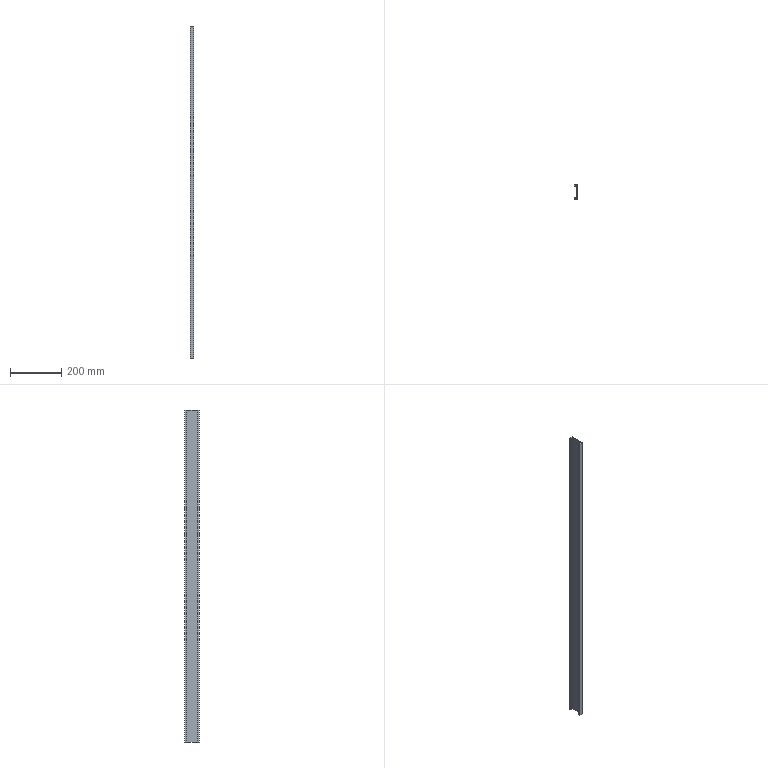Part | STEP file | Guide wheel mechanism revised.sldasm-Part-330 | 1 solid | 14 faces | box 12 x 56 x 1300 mm | volume 319800 mm3 | plane 14
STEP:
#1=CARTESIAN_POINT('',(3.,-25.,-650.));
#2=VERTEX_POINT('',#1);
#3=CARTESIAN_POINT('',(-3.,-25.,-650.));
#4=VERTEX_POINT('',#3);
#5=CARTESIAN_POINT('',(-3.,-25.,-650.));
#6=DIRECTION('',(-1.,0.,0.));
#7=VECTOR('',#6,1000.);
#8=LINE('',#5,#7);
#9=EDGE_CURVE('',#2,#4,#8,.T.);
#10=ORIENTED_EDGE('',*,*,#9,.T.);
#11=CARTESIAN_POINT('',(-3.,-25.,650.));
#12=VERTEX_POINT('',#11);
#13=CARTESIAN_POINT('',(-3.,-25.,650.));
#14=DIRECTION('',(0.,0.,-1.));
#15=VECTOR('',#14,1000.);
#16=LINE('',#13,#15);
#17=EDGE_CURVE('',#12,#4,#16,.T.);
#18=ORIENTED_EDGE('',*,*,#17,.F.);
#19=CARTESIAN_POINT('',(3.,-25.,650.));
#20=VERTEX_POINT('',#19);
#21=CARTESIAN_POINT('',(-3.,-25.,650.));
#22=DIRECTION('',(-1.,0.,0.));
#23=VECTOR('',#22,1000.);
#24=LINE('',#21,#23);
#25=EDGE_CURVE('',#20,#12,#24,.T.);
#26=ORIENTED_EDGE('',*,*,#25,.F.);
#27=CARTESIAN_POINT('',(3.,-25.,650.));
#28=DIRECTION('',(0.,0.,-1.));
#29=VECTOR('',#28,1000.);
#30=LINE('',#27,#29);
#31=EDGE_CURVE('',#20,#2,#30,.T.);
#32=ORIENTED_EDGE('',*,*,#31,.T.);
#33=EDGE_LOOP('',(#10,#18,#26,#32));
#34=FACE_OUTER_BOUND('',#33,.T.);
#35=CARTESIAN_POINT('',(-3.,-25.,650.));
#36=DIRECTION('',(0.,-1.,0.));
#37=DIRECTION('',(0.,0.,-1.));
#38=AXIS2_PLACEMENT_3D('',#35,#36,#37);
#39=PLANE('',#38);
#40=ADVANCED_FACE('',(#34),#39,.F.);
#41=CARTESIAN_POINT('',(-3.,-21.,-650.));
#42=VERTEX_POINT('',#41);
#43=CARTESIAN_POINT('',(-3.,-21.,-650.));
#44=DIRECTION('',(0.,1.,0.));
#45=VECTOR('',#44,1000.);
#46=LINE('',#43,#45);
#47=EDGE_CURVE('',#4,#42,#46,.T.);
#48=ORIENTED_EDGE('',*,*,#47,.T.);
#49=CARTESIAN_POINT('',(-3.,-21.,650.));
#50=VERTEX_POINT('',#49);
#51=CARTESIAN_POINT('',(-3.,-21.,650.));
#52=DIRECTION('',(0.,0.,-1.));
#53=VECTOR('',#52,1000.);
#54=LINE('',#51,#53);
#55=EDGE_CURVE('',#50,#42,#54,.T.);
#56=ORIENTED_EDGE('',*,*,#55,.F.);
#57=CARTESIAN_POINT('',(-3.,-21.,650.));
#58=DIRECTION('',(0.,1.,0.));
#59=VECTOR('',#58,1000.);
#60=LINE('',#57,#59);
#61=EDGE_CURVE('',#12,#50,#60,.T.);
#62=ORIENTED_EDGE('',*,*,#61,.F.);
#63=ORIENTED_EDGE('',*,*,#17,.T.);
#64=EDGE_LOOP('',(#48,#56,#62,#63));
#65=FACE_OUTER_BOUND('',#64,.T.);
#66=CARTESIAN_POINT('',(-3.,-21.,650.));
#67=DIRECTION('',(-1.,0.,0.));
#68=DIRECTION('',(0.,0.,1.));
#69=AXIS2_PLACEMENT_3D('',#66,#67,#68);
#70=PLANE('',#69);
#71=ADVANCED_FACE('',(#65),#70,.F.);
#72=CARTESIAN_POINT('',(-6.,-21.,-650.));
#73=VERTEX_POINT('',#72);
#74=CARTESIAN_POINT('',(-3.,-21.,-650.));
#75=DIRECTION('',(-1.,0.,0.));
#76=VECTOR('',#75,1000.);
#77=LINE('',#74,#76);
#78=EDGE_CURVE('',#42,#73,#77,.T.);
#79=ORIENTED_EDGE('',*,*,#78,.T.);
#80=CARTESIAN_POINT('',(-6.,-21.,650.));
#81=VERTEX_POINT('',#80);
#82=CARTESIAN_POINT('',(-6.,-21.,650.));
#83=DIRECTION('',(0.,0.,-1.));
#84=VECTOR('',#83,1000.);
#85=LINE('',#82,#84);
#86=EDGE_CURVE('',#81,#73,#85,.T.);
#87=ORIENTED_EDGE('',*,*,#86,.F.);
#88=CARTESIAN_POINT('',(-3.,-21.,650.));
#89=DIRECTION('',(-1.,0.,0.));
#90=VECTOR('',#89,1000.);
#91=LINE('',#88,#90);
#92=EDGE_CURVE('',#50,#81,#91,.T.);
#93=ORIENTED_EDGE('',*,*,#92,.F.);
#94=ORIENTED_EDGE('',*,*,#55,.T.);
#95=EDGE_LOOP('',(#79,#87,#93,#94));
#96=FACE_OUTER_BOUND('',#95,.T.);
#97=CARTESIAN_POINT('',(-3.,-21.,650.));
#98=DIRECTION('',(0.,-1.,0.));
#99=DIRECTION('',(0.,0.,-1.));
#100=AXIS2_PLACEMENT_3D('',#97,#98,#99);
#101=PLANE('',#100);
#102=ADVANCED_FACE('',(#96),#101,.F.);
#103=CARTESIAN_POINT('',(-6.,-28.,-650.));
#104=VERTEX_POINT('',#103);
#105=CARTESIAN_POINT('',(-6.,-21.,-650.));
#106=DIRECTION('',(0.,-1.,0.));
#107=VECTOR('',#106,1000.);
#108=LINE('',#105,#107);
#109=EDGE_CURVE('',#73,#104,#108,.T.);
#110=ORIENTED_EDGE('',*,*,#109,.T.);
#111=CARTESIAN_POINT('',(-6.,-28.,650.));
#112=VERTEX_POINT('',#111);
#113=CARTESIAN_POINT('',(-6.,-28.,650.));
#114=DIRECTION('',(0.,0.,-1.));
#115=VECTOR('',#114,1000.);
#116=LINE('',#113,#115);
#117=EDGE_CURVE('',#112,#104,#116,.T.);
#118=ORIENTED_EDGE('',*,*,#117,.F.);
#119=CARTESIAN_POINT('',(-6.,-21.,650.));
#120=DIRECTION('',(0.,-1.,0.));
#121=VECTOR('',#120,1000.);
#122=LINE('',#119,#121);
#123=EDGE_CURVE('',#81,#112,#122,.T.);
#124=ORIENTED_EDGE('',*,*,#123,.F.);
#125=ORIENTED_EDGE('',*,*,#86,.T.);
#126=EDGE_LOOP('',(#110,#118,#124,#125));
#127=FACE_OUTER_BOUND('',#126,.T.);
#128=CARTESIAN_POINT('',(-6.,-21.,650.));
#129=DIRECTION('',(1.,0.,0.));
#130=DIRECTION('',(0.,0.,-1.));
#131=AXIS2_PLACEMENT_3D('',#128,#129,#130);
#132=PLANE('',#131);
#133=ADVANCED_FACE('',(#127),#132,.F.);
#134=CARTESIAN_POINT('',(6.,-28.,-650.));
#135=VERTEX_POINT('',#134);
#136=CARTESIAN_POINT('',(-6.,-28.,-650.));
#137=DIRECTION('',(1.,0.,0.));
#138=VECTOR('',#137,1000.);
#139=LINE('',#136,#138);
#140=EDGE_CURVE('',#104,#135,#139,.T.);
#141=ORIENTED_EDGE('',*,*,#140,.T.);
#142=CARTESIAN_POINT('',(6.,-28.,650.));
#143=VERTEX_POINT('',#142);
#144=CARTESIAN_POINT('',(6.,-28.,650.));
#145=DIRECTION('',(0.,0.,-1.));
#146=VECTOR('',#145,1000.);
#147=LINE('',#144,#146);
#148=EDGE_CURVE('',#143,#135,#147,.T.);
#149=ORIENTED_EDGE('',*,*,#148,.F.);
#150=CARTESIAN_POINT('',(-6.,-28.,650.));
#151=DIRECTION('',(1.,0.,0.));
#152=VECTOR('',#151,1000.);
#153=LINE('',#150,#152);
#154=EDGE_CURVE('',#112,#143,#153,.T.);
#155=ORIENTED_EDGE('',*,*,#154,.F.);
#156=ORIENTED_EDGE('',*,*,#117,.T.);
#157=EDGE_LOOP('',(#141,#149,#155,#156));
#158=FACE_OUTER_BOUND('',#157,.T.);
#159=CARTESIAN_POINT('',(-6.,-28.,650.));
#160=DIRECTION('',(0.,1.,0.));
#161=DIRECTION('',(0.,0.,1.));
#162=AXIS2_PLACEMENT_3D('',#159,#160,#161);
#163=PLANE('',#162);
#164=ADVANCED_FACE('',(#158),#163,.F.);
#165=CARTESIAN_POINT('',(6.,28.,-650.));
#166=VERTEX_POINT('',#165);
#167=CARTESIAN_POINT('',(6.,-28.,-650.));
#168=DIRECTION('',(0.,1.,0.));
#169=VECTOR('',#168,1000.);
#170=LINE('',#167,#169);
#171=EDGE_CURVE('',#135,#166,#170,.T.);
#172=ORIENTED_EDGE('',*,*,#171,.T.);
#173=CARTESIAN_POINT('',(6.,28.,650.));
#174=VERTEX_POINT('',#173);
#175=CARTESIAN_POINT('',(6.,28.,650.));
#176=DIRECTION('',(0.,0.,-1.));
#177=VECTOR('',#176,1000.);
#178=LINE('',#175,#177);
#179=EDGE_CURVE('',#174,#166,#178,.T.);
#180=ORIENTED_EDGE('',*,*,#179,.F.);
#181=CARTESIAN_POINT('',(6.,-28.,650.));
#182=DIRECTION('',(0.,1.,0.));
#183=VECTOR('',#182,1000.);
#184=LINE('',#181,#183);
#185=EDGE_CURVE('',#143,#174,#184,.T.);
#186=ORIENTED_EDGE('',*,*,#185,.F.);
#187=ORIENTED_EDGE('',*,*,#148,.T.);
#188=EDGE_LOOP('',(#172,#180,#186,#187));
#189=FACE_OUTER_BOUND('',#188,.T.);
#190=CARTESIAN_POINT('',(6.,-28.,650.));
#191=DIRECTION('',(-1.,0.,0.));
#192=DIRECTION('',(0.,0.,1.));
#193=AXIS2_PLACEMENT_3D('',#190,#191,#192);
#194=PLANE('',#193);
#195=ADVANCED_FACE('',(#189),#194,.F.);
#196=CARTESIAN_POINT('',(-6.,28.,-650.));
#197=VERTEX_POINT('',#196);
#198=CARTESIAN_POINT('',(6.,28.,-650.));
#199=DIRECTION('',(-1.,0.,0.));
#200=VECTOR('',#199,1000.);
#201=LINE('',#198,#200);
#202=EDGE_CURVE('',#166,#197,#201,.T.);
#203=ORIENTED_EDGE('',*,*,#202,.T.);
#204=CARTESIAN_POINT('',(-6.,28.,650.));
#205=VERTEX_POINT('',#204);
#206=CARTESIAN_POINT('',(-6.,28.,650.));
#207=DIRECTION('',(0.,0.,-1.));
#208=VECTOR('',#207,1000.);
#209=LINE('',#206,#208);
#210=EDGE_CURVE('',#205,#197,#209,.T.);
#211=ORIENTED_EDGE('',*,*,#210,.F.);
#212=CARTESIAN_POINT('',(6.,28.,650.));
#213=DIRECTION('',(-1.,0.,0.));
#214=VECTOR('',#213,1000.);
#215=LINE('',#212,#214);
#216=EDGE_CURVE('',#174,#205,#215,.T.);
#217=ORIENTED_EDGE('',*,*,#216,.F.);
#218=ORIENTED_EDGE('',*,*,#179,.T.);
#219=EDGE_LOOP('',(#203,#211,#217,#218));
#220=FACE_OUTER_BOUND('',#219,.T.);
#221=CARTESIAN_POINT('',(6.,28.,650.));
#222=DIRECTION('',(0.,-1.,0.));
#223=DIRECTION('',(1.,0.,0.));
#224=AXIS2_PLACEMENT_3D('',#221,#222,#223);
#225=PLANE('',#224);
#226=ADVANCED_FACE('',(#220),#225,.F.);
#227=CARTESIAN_POINT('',(-6.,21.,-650.));
#228=VERTEX_POINT('',#227);
#229=CARTESIAN_POINT('',(-6.,28.,-650.));
#230=DIRECTION('',(0.,-1.,0.));
#231=VECTOR('',#230,1000.);
#232=LINE('',#229,#231);
#233=EDGE_CURVE('',#197,#228,#232,.T.);
#234=ORIENTED_EDGE('',*,*,#233,.T.);
#235=CARTESIAN_POINT('',(-6.,21.,650.));
#236=VERTEX_POINT('',#235);
#237=CARTESIAN_POINT('',(-6.,21.,650.));
#238=DIRECTION('',(0.,0.,-1.));
#239=VECTOR('',#238,1000.);
#240=LINE('',#237,#239);
#241=EDGE_CURVE('',#236,#228,#240,.T.);
#242=ORIENTED_EDGE('',*,*,#241,.F.);
#243=CARTESIAN_POINT('',(-6.,28.,650.));
#244=DIRECTION('',(0.,-1.,0.));
#245=VECTOR('',#244,1000.);
#246=LINE('',#243,#245);
#247=EDGE_CURVE('',#205,#236,#246,.T.);
#248=ORIENTED_EDGE('',*,*,#247,.F.);
#249=ORIENTED_EDGE('',*,*,#210,.T.);
#250=EDGE_LOOP('',(#234,#242,#248,#249));
#251=FACE_OUTER_BOUND('',#250,.T.);
#252=CARTESIAN_POINT('',(-6.,28.,650.));
#253=DIRECTION('',(1.,0.,0.));
#254=DIRECTION('',(0.,1.,0.));
#255=AXIS2_PLACEMENT_3D('',#252,#253,#254);
#256=PLANE('',#255);
#257=ADVANCED_FACE('',(#251),#256,.F.);
#258=CARTESIAN_POINT('',(-3.,21.,-650.));
#259=VERTEX_POINT('',#258);
#260=CARTESIAN_POINT('',(-3.,21.,-650.));
#261=DIRECTION('',(1.,0.,0.));
#262=VECTOR('',#261,1000.);
#263=LINE('',#260,#262);
#264=EDGE_CURVE('',#228,#259,#263,.T.);
#265=ORIENTED_EDGE('',*,*,#264,.T.);
#266=CARTESIAN_POINT('',(-3.,21.,650.));
#267=VERTEX_POINT('',#266);
#268=CARTESIAN_POINT('',(-3.,21.,650.));
#269=DIRECTION('',(0.,0.,-1.));
#270=VECTOR('',#269,1000.);
#271=LINE('',#268,#270);
#272=EDGE_CURVE('',#267,#259,#271,.T.);
#273=ORIENTED_EDGE('',*,*,#272,.F.);
#274=CARTESIAN_POINT('',(-3.,21.,650.));
#275=DIRECTION('',(1.,0.,0.));
#276=VECTOR('',#275,1000.);
#277=LINE('',#274,#276);
#278=EDGE_CURVE('',#236,#267,#277,.T.);
#279=ORIENTED_EDGE('',*,*,#278,.F.);
#280=ORIENTED_EDGE('',*,*,#241,.T.);
#281=EDGE_LOOP('',(#265,#273,#279,#280));
#282=FACE_OUTER_BOUND('',#281,.T.);
#283=CARTESIAN_POINT('',(-3.,21.,650.));
#284=DIRECTION('',(0.,1.,0.));
#285=DIRECTION('',(0.,0.,1.));
#286=AXIS2_PLACEMENT_3D('',#283,#284,#285);
#287=PLANE('',#286);
#288=ADVANCED_FACE('',(#282),#287,.F.);
#289=CARTESIAN_POINT('',(-3.,25.,-650.));
#290=VERTEX_POINT('',#289);
#291=CARTESIAN_POINT('',(-3.,25.,-650.));
#292=DIRECTION('',(0.,1.,0.));
#293=VECTOR('',#292,1000.);
#294=LINE('',#291,#293);
#295=EDGE_CURVE('',#259,#290,#294,.T.);
#296=ORIENTED_EDGE('',*,*,#295,.T.);
#297=CARTESIAN_POINT('',(-3.,25.,650.));
#298=VERTEX_POINT('',#297);
#299=CARTESIAN_POINT('',(-3.,25.,650.));
#300=DIRECTION('',(0.,0.,-1.));
#301=VECTOR('',#300,1000.);
#302=LINE('',#299,#301);
#303=EDGE_CURVE('',#298,#290,#302,.T.);
#304=ORIENTED_EDGE('',*,*,#303,.F.);
#305=CARTESIAN_POINT('',(-3.,25.,650.));
#306=DIRECTION('',(0.,1.,0.));
#307=VECTOR('',#306,1000.);
#308=LINE('',#305,#307);
#309=EDGE_CURVE('',#267,#298,#308,.T.);
#310=ORIENTED_EDGE('',*,*,#309,.F.);
#311=ORIENTED_EDGE('',*,*,#272,.T.);
#312=EDGE_LOOP('',(#296,#304,#310,#311));
#313=FACE_OUTER_BOUND('',#312,.T.);
#314=CARTESIAN_POINT('',(-3.,25.,650.));
#315=DIRECTION('',(-1.,0.,0.));
#316=DIRECTION('',(0.,0.,1.));
#317=AXIS2_PLACEMENT_3D('',#314,#315,#316);
#318=PLANE('',#317);
#319=ADVANCED_FACE('',(#313),#318,.F.);
#320=CARTESIAN_POINT('',(3.,25.,-650.));
#321=VERTEX_POINT('',#320);
#322=CARTESIAN_POINT('',(3.,25.,-650.));
#323=DIRECTION('',(1.,0.,0.));
#324=VECTOR('',#323,1000.);
#325=LINE('',#322,#324);
#326=EDGE_CURVE('',#290,#321,#325,.T.);
#327=ORIENTED_EDGE('',*,*,#326,.T.);
#328=CARTESIAN_POINT('',(3.,25.,650.));
#329=VERTEX_POINT('',#328);
#330=CARTESIAN_POINT('',(3.,25.,650.));
#331=DIRECTION('',(0.,0.,-1.));
#332=VECTOR('',#331,1000.);
#333=LINE('',#330,#332);
#334=EDGE_CURVE('',#329,#321,#333,.T.);
#335=ORIENTED_EDGE('',*,*,#334,.F.);
#336=CARTESIAN_POINT('',(3.,25.,650.));
#337=DIRECTION('',(1.,0.,0.));
#338=VECTOR('',#337,1000.);
#339=LINE('',#336,#338);
#340=EDGE_CURVE('',#298,#329,#339,.T.);
#341=ORIENTED_EDGE('',*,*,#340,.F.);
#342=ORIENTED_EDGE('',*,*,#303,.T.);
#343=EDGE_LOOP('',(#327,#335,#341,#342));
#344=FACE_OUTER_BOUND('',#343,.T.);
#345=CARTESIAN_POINT('',(3.,25.,650.));
#346=DIRECTION('',(0.,1.,0.));
#347=DIRECTION('',(0.,0.,1.));
#348=AXIS2_PLACEMENT_3D('',#345,#346,#347);
#349=PLANE('',#348);
#350=ADVANCED_FACE('',(#344),#349,.F.);
#351=CARTESIAN_POINT('',(3.,-25.,-650.));
#352=DIRECTION('',(0.,-1.,0.));
#353=VECTOR('',#352,1000.);
#354=LINE('',#351,#353);
#355=EDGE_CURVE('',#321,#2,#354,.T.);
#356=ORIENTED_EDGE('',*,*,#355,.T.);
#357=ORIENTED_EDGE('',*,*,#31,.F.);
#358=CARTESIAN_POINT('',(3.,-25.,650.));
#359=DIRECTION('',(0.,-1.,0.));
#360=VECTOR('',#359,1000.);
#361=LINE('',#358,#360);
#362=EDGE_CURVE('',#329,#20,#361,.T.);
#363=ORIENTED_EDGE('',*,*,#362,.F.);
#364=ORIENTED_EDGE('',*,*,#334,.T.);
#365=EDGE_LOOP('',(#356,#357,#363,#364));
#366=FACE_OUTER_BOUND('',#365,.T.);
#367=CARTESIAN_POINT('',(3.,-25.,650.));
#368=DIRECTION('',(1.,0.,0.));
#369=DIRECTION('',(0.,0.,-1.));
#370=AXIS2_PLACEMENT_3D('',#367,#368,#369);
#371=PLANE('',#370);
#372=ADVANCED_FACE('',(#366),#371,.F.);
#373=ORIENTED_EDGE('',*,*,#25,.T.);
#374=ORIENTED_EDGE('',*,*,#61,.T.);
#375=ORIENTED_EDGE('',*,*,#92,.T.);
#376=ORIENTED_EDGE('',*,*,#123,.T.);
#377=ORIENTED_EDGE('',*,*,#154,.T.);
#378=ORIENTED_EDGE('',*,*,#185,.T.);
#379=ORIENTED_EDGE('',*,*,#216,.T.);
#380=ORIENTED_EDGE('',*,*,#247,.T.);
#381=ORIENTED_EDGE('',*,*,#278,.T.);
#382=ORIENTED_EDGE('',*,*,#309,.T.);
#383=ORIENTED_EDGE('',*,*,#340,.T.);
#384=ORIENTED_EDGE('',*,*,#362,.T.);
#385=EDGE_LOOP('',(#373,#374,#375,#376,#377,#378,#379,#380,#381,#382,#383,#384));
#386=FACE_OUTER_BOUND('',#385,.T.);
#387=CARTESIAN_POINT('',(0.,0.,650.));
#388=DIRECTION('',(0.,0.,1.));
#389=DIRECTION('',(1.,0.,0.));
#390=AXIS2_PLACEMENT_3D('',#387,#388,#389);
#391=PLANE('',#390);
#392=ADVANCED_FACE('',(#386),#391,.T.);
#393=ORIENTED_EDGE('',*,*,#9,.F.);
#394=ORIENTED_EDGE('',*,*,#355,.F.);
#395=ORIENTED_EDGE('',*,*,#326,.F.);
#396=ORIENTED_EDGE('',*,*,#295,.F.);
#397=ORIENTED_EDGE('',*,*,#264,.F.);
#398=ORIENTED_EDGE('',*,*,#233,.F.);
#399=ORIENTED_EDGE('',*,*,#202,.F.);
#400=ORIENTED_EDGE('',*,*,#171,.F.);
#401=ORIENTED_EDGE('',*,*,#140,.F.);
#402=ORIENTED_EDGE('',*,*,#109,.F.);
#403=ORIENTED_EDGE('',*,*,#78,.F.);
#404=ORIENTED_EDGE('',*,*,#47,.F.);
#405=EDGE_LOOP('',(#393,#394,#395,#396,#397,#398,#399,#400,#401,#402,#403,#404));
#406=FACE_OUTER_BOUND('',#405,.T.);
#407=CARTESIAN_POINT('',(0.,0.,-650.));
#408=DIRECTION('',(0.,0.,1.));
#409=DIRECTION('',(1.,0.,0.));
#410=AXIS2_PLACEMENT_3D('',#407,#408,#409);
#411=PLANE('',#410);
#412=ADVANCED_FACE('',(#406),#411,.F.);
#413=CLOSED_SHELL('',(#40,#71,#102,#133,#164,#195,#226,#257,#288,#319,#350,#372,#392,#412));
#414=MANIFOLD_SOLID_BREP('',#413);
#415=CARTESIAN_POINT('',(0.,0.,0.));
#416=DIRECTION('',(0.,0.,1.));
#417=DIRECTION('',(1.,0.,0.));
#418=AXIS2_PLACEMENT_3D('',#415,#416,#417);
#419=(LENGTH_UNIT()NAMED_UNIT(*)SI_UNIT(.MILLI.,.METRE.));
#420=UNCERTAINTY_MEASURE_WITH_UNIT(LENGTH_MEASURE(0.00001),#419,'','');
#421=(NAMED_UNIT(*)PLANE_ANGLE_UNIT()SI_UNIT($,.RADIAN.));
#422=(NAMED_UNIT(*)SI_UNIT($,.STERADIAN.)SOLID_ANGLE_UNIT());
#423=(GEOMETRIC_REPRESENTATION_CONTEXT(3)GLOBAL_UNCERTAINTY_ASSIGNED_CONTEXT((#420))GLOBAL_UNIT_ASSIGNED_CONTEXT((#419,#421,#422))REPRESENTATION_CONTEXT('',''));
#424=ADVANCED_BREP_SHAPE_REPRESENTATION('',(#414,#418),#423);